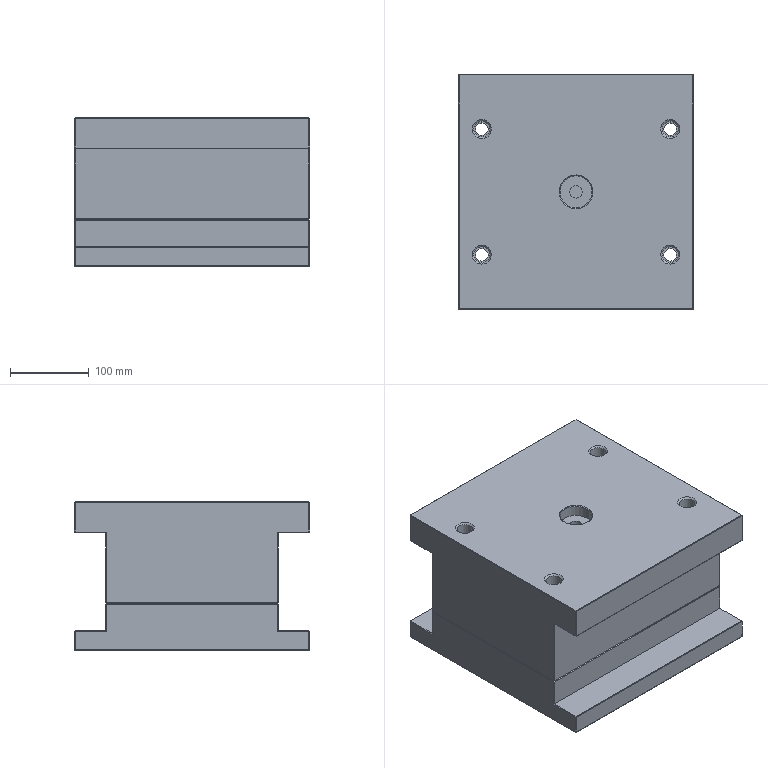NC program | NX | posted with a generic post | part box 300 x 300 x 190 mm
Lines 1 to 721 of 1853:
N10 G17 G21 G94 G90
(HOLE_MILLING_COPY_2 , TOOL : D10C)
N12 T10 M6
N14 G54
N16 G17 G0 G90 X-120. Y80. S2000 M3
N18 G43 Z30. H10
N20 Z0.5
N22 G94 G3 X-117.5 Y77.5 R2.5 F800.
N24 X-115. Y80. R2.5
N26 X-115. Y80. Z0.3 I-5. J0.
N28 X-115. Y80. Z0.1 I-5. J0.
N30 X-115. Y80. Z-0.1 I-5. J0.
N32 X-115. Y80. Z-0.3 I-5. J0.
N34 X-115. Y80. Z-0.5 I-5. J0.
N36 X-115. Y80. Z-0.7 I-5. J0.
N38 X-115. Y80. Z-0.9 I-5. J0.
N40 X-115. Y80. Z-1.1 I-5. J0.
N42 X-115. Y80. Z-1.3 I-5. J0.
N44 X-115. Y80. Z-1.5 I-5. J0.
N46 X-115. Y80. Z-1.7 I-5. J0.
N48 X-115. Y80. Z-1.9 I-5. J0.
N50 X-115. Y80. Z-2.1 I-5. J0.
N52 X-115. Y80. Z-2.3 I-5. J0.
N54 X-115. Y80. Z-2.5 I-5. J0.
N56 X-115. Y80. Z-2.7 I-5. J0.
N58 X-115. Y80. Z-2.9 I-5. J0.
N60 X-115. Y80. Z-3.1 I-5. J0.
N62 X-115. Y80. Z-3.3 I-5. J0.
N64 X-115. Y80. Z-3.5 I-5. J0.
N66 X-115. Y80. Z-3.7 I-5. J0.
N68 X-115. Y80. Z-3.9 I-5. J0.
N70 X-115. Y80. Z-4.1 I-5. J0.
N72 X-115. Y80. Z-4.3 I-5. J0.
N74 X-115. Y80. Z-4.5 I-5. J0.
N76 X-115. Y80. Z-4.7 I-5. J0.
N78 X-115. Y80. Z-4.9 I-5. J0.
N80 X-115. Y80. Z-5.1 I-5. J0.
N82 X-115. Y80. Z-5.3 I-5. J0.
N84 X-115. Y80. Z-5.5 I-5. J0.
N86 X-115. Y80. Z-5.7 I-5. J0.
N88 X-115. Y80. Z-5.9 I-5. J0.
N90 X-115. Y80. Z-6.1 I-5. J0.
N92 X-115. Y80. Z-6.3 I-5. J0.
N94 X-115. Y80. Z-6.5 I-5. J0.
N96 X-115. Y80. Z-6.7 I-5. J0.
N98 X-115. Y80. Z-6.9 I-5. J0.
N100 X-115. Y80. Z-7.1 I-5. J0.
N102 X-115. Y80. Z-7.3 I-5. J0.
N104 X-115. Y80. Z-7.5 I-5. J0.
N106 X-115. Y80. Z-7.7 I-5. J0.
N108 X-115. Y80. Z-7.9 I-5. J0.
N110 X-115. Y80. Z-8.1 I-5. J0.
N112 X-115. Y80. Z-8.3 I-5. J0.
N114 X-115. Y80. Z-8.5 I-5. J0.
N116 X-115. Y80. Z-8.7 I-5. J0.
N118 X-115. Y80. Z-8.9 I-5. J0.
N120 X-115. Y80. Z-9.1 I-5. J0.
N122 X-115. Y80. Z-9.3 I-5. J0.
N124 X-115. Y80. Z-9.5 I-5. J0.
N126 X-115. Y80. Z-9.7 I-5. J0.
N128 X-115. Y80. Z-9.9 I-5. J0.
N130 X-115. Y80. Z-10.1 I-5. J0.
N132 X-115. Y80. Z-10.3 I-5. J0.
N134 X-115. Y80. Z-10.5 I-5. J0.
N136 X-115. Y80. Z-10.7 I-5. J0.
N138 X-115. Y80. Z-10.9 I-5. J0.
N140 X-115. Y80. Z-11.1 I-5. J0.
N142 X-115. Y80. Z-11.3 I-5. J0.
N144 X-115. Y80. Z-11.5 I-5. J0.
N146 X-115. Y80. Z-11.7 I-5. J0.
N148 X-115. Y80. Z-11.9 I-5. J0.
N150 X-115. Y80. Z-12.1 I-5. J0.
N152 X-115. Y80. Z-12.3 I-5. J0.
N154 X-115. Y80. Z-12.5 I-5. J0.
N156 X-115. Y80. Z-12.7 I-5. J0.
N158 X-115. Y80. Z-12.9 I-5. J0.
N160 X-115. Y80. Z-13.1 I-5. J0.
N162 X-115. Y80. Z-13.3 I-5. J0.
N164 X-115. Y80. Z-13.5 I-5. J0.
N166 X-115. Y80. Z-13.7 I-5. J0.
N168 X-115. Y80. Z-13.9 I-5. J0.
N170 X-115. Y80. Z-14.1 I-5. J0.
N172 X-115. Y80. Z-14.3 I-5. J0.
N174 X-115. Y80. Z-14.5 I-5. J0.
N176 X-115. Y80. Z-14.7 I-5. J0.
N178 X-115. Y80. Z-14.9 I-5. J0.
N180 X-115. Y80. Z-15.1 I-5. J0.
N182 X-115. Y80. Z-15.3 I-5. J0.
N184 X-115. Y80. Z-15.5 I-5. J0.
N186 X-115. Y80. Z-15.7 I-5. J0.
N188 X-115. Y80. Z-15.9 I-5. J0.
N190 X-115. Y80. Z-16.1 I-5. J0.
N192 X-115. Y80. Z-16.3 I-5. J0.
N194 X-115. Y80. Z-16.5 I-5. J0.
N196 X-115. Y80. Z-16.7 I-5. J0.
N198 X-115. Y80. Z-16.9 I-5. J0.
N200 X-115. Y80. Z-17.1 I-5. J0.
N202 X-115. Y80. Z-17.3 I-5. J0.
N204 X-115. Y80. Z-17.5 I-5. J0.
N206 X-115. Y80. Z-17.7 I-5. J0.
N208 X-115. Y80. Z-17.9 I-5. J0.
N210 X-115. Y80. Z-18.1 I-5. J0.
N212 X-115. Y80. Z-18.3 I-5. J0.
N214 X-115. Y80. Z-18.5 I-5. J0.
N216 X-115. Y80. Z-18.7 I-5. J0.
N218 X-115. Y80. Z-18.9 I-5. J0.
N220 X-115. Y80. Z-19.1 I-5. J0.
N222 X-115. Y80. Z-19.3 I-5. J0.
N224 X-115. Y80. Z-19.5 I-5. J0.
N226 X-115. Y80. Z-19.7 I-5. J0.
N228 X-115. Y80. Z-19.9 I-5. J0.
N230 X-115. Y80. Z-20.1 I-5. J0.
N232 X-115. Y80. Z-20.3 I-5. J0.
N234 X-115. Y80. Z-20.5 I-5. J0.
N236 X-115. Y80. Z-20.7 I-5. J0.
N238 X-115. Y80. Z-20.9 I-5. J0.
N240 X-115. Y80. Z-21.1 I-5. J0.
N242 X-115. Y80. Z-21.3 I-5. J0.
N244 X-115. Y80. Z-21.5 I-5. J0.
N246 X-115. Y80. Z-21.7 I-5. J0.
N248 X-115. Y80. Z-21.9 I-5. J0.
N250 X-115. Y80. Z-22.1 I-5. J0.
N252 X-115. Y80. Z-22.3 I-5. J0.
N254 X-115. Y80. Z-22.5 I-5. J0.
N256 X-115. Y80. Z-22.7 I-5. J0.
N258 X-115. Y80. Z-22.9 I-5. J0.
N260 X-115. Y80. Z-23.1 I-5. J0.
N262 X-115. Y80. Z-23.3 I-5. J0.
N264 X-115. Y80. Z-23.5 I-5. J0.
N266 X-115. Y80. Z-23.7 I-5. J0.
N268 X-115. Y80. Z-23.9 I-5. J0.
N270 X-115. Y80. Z-24.1 I-5. J0.
N272 X-115. Y80. Z-24.3 I-5. J0.
N274 X-115. Y80. Z-24.5 I-5. J0.
N276 X-115. Y80. Z-24.7 I-5. J0.
N278 X-115. Y80. Z-24.9 I-5. J0.
N280 X-115. Y80. Z-25.1 I-5. J0.
N282 X-115. Y80. Z-25.3 I-5. J0.
N284 X-115. Y80. Z-25.5 I-5. J0.
N286 X-115. Y80. Z-25.7 I-5. J0.
N288 X-115. Y80. Z-25.9 I-5. J0.
N290 X-115. Y80. Z-26.1 I-5. J0.
N292 X-115. Y80. Z-26.3 I-5. J0.
N294 X-115. Y80. Z-26.5 I-5. J0.
N296 X-115. Y80. Z-26.7 I-5. J0.
N298 X-115. Y80. Z-26.9 I-5. J0.
N300 X-115. Y80. Z-27.1 I-5. J0.
N302 X-115. Y80. Z-27.3 I-5. J0.
N304 X-115. Y80. Z-27.5 I-5. J0.
N306 X-115. Y80. Z-27.7 I-5. J0.
N308 X-115. Y80. Z-27.9 I-5. J0.
N310 X-115. Y80. Z-28.1 I-5. J0.
N312 X-115. Y80. Z-28.3 I-5. J0.
N314 X-115. Y80. Z-28.5 I-5. J0.
N316 X-115. Y80. Z-28.7 I-5. J0.
N318 X-115. Y80. Z-28.9 I-5. J0.
N320 X-115. Y80. Z-29.1 I-5. J0.
N322 X-115. Y80. Z-29.3 I-5. J0.
N324 X-115. Y80. Z-29.5 I-5. J0.
N326 X-115. Y80. Z-29.7 I-5. J0.
N328 X-115. Y80. Z-29.9 I-5. J0.
N330 X-115. Y80. Z-30.1 I-5. J0.
N332 X-115. Y80. Z-30.3 I-5. J0.
N334 X-115. Y80. Z-30.5 I-5. J0.
N336 X-115. Y80. Z-30.7 I-5. J0.
N338 X-115. Y80. Z-30.9 I-5. J0.
N340 X-115. Y80. Z-31.1 I-5. J0.
N342 X-115. Y80. Z-31.3 I-5. J0.
N344 X-115. Y80. Z-31.5 I-5. J0.
N346 X-115. Y80. Z-31.7 I-5. J0.
N348 X-115. Y80. Z-31.9 I-5. J0.
N350 X-115. Y80. Z-32.1 I-5. J0.
N352 X-115. Y80. Z-32.3 I-5. J0.
N354 X-115. Y80. Z-32.5 I-5. J0.
N356 X-115. Y80. Z-32.7 I-5. J0.
N358 X-115. Y80. Z-32.9 I-5. J0.
N360 X-115. Y80. Z-33.1 I-5. J0.
N362 X-115. Y80. Z-33.3 I-5. J0.
N364 X-115. Y80. Z-33.5 I-5. J0.
N366 X-115. Y80. Z-33.7 I-5. J0.
N368 X-115. Y80. Z-33.9 I-5. J0.
N370 X-115. Y80. Z-34.1 I-5. J0.
N372 X-115. Y80. Z-34.3 I-5. J0.
N374 X-115. Y80. Z-34.5 I-5. J0.
N376 X-115. Y80. Z-34.7 I-5. J0.
N378 X-115. Y80. Z-34.9 I-5. J0.
N380 X-115. Y80. Z-35.1 I-5. J0.
N382 X-115. Y80. Z-35.3 I-5. J0.
N384 X-115. Y80. Z-35.5 I-5. J0.
N386 X-115. Y80. Z-35.7 I-5. J0.
N388 X-115. Y80. Z-35.9 I-5. J0.
N390 X-115. Y80. Z-36.1 I-5. J0.
N392 X-115. Y80. Z-36.3 I-5. J0.
N394 X-115. Y80. Z-36.5 I-5. J0.
N396 X-115. Y80. Z-36.7 I-5. J0.
N398 X-115. Y80. Z-36.9 I-5. J0.
N400 X-115. Y80. Z-37.1 I-5. J0.
N402 X-115. Y80. Z-37.3 I-5. J0.
N404 X-115. Y80. Z-37.5 I-5. J0.
N406 X-115. Y80. Z-37.7 I-5. J0.
N408 X-115. Y80. Z-37.9 I-5. J0.
N410 X-115. Y80. Z-38.1 I-5. J0.
N412 X-115. Y80. Z-38.3 I-5. J0.
N414 X-115. Y80. Z-38.5 I-5. J0.
N416 X-115. Y80. Z-38.7 I-5. J0.
N418 X-115. Y80. Z-38.9 I-5. J0.
N420 X-115. Y80. Z-39.1 I-5. J0.
N422 X-115. Y80. Z-39.3 I-5. J0.
N424 X-115. Y80. Z-39.5 I-5. J0.
N426 X-115. Y80. Z-39.7 I-5. J0.
N428 X-115. Y80. Z-39.9 I-5. J0.
N430 X-115. Y80. Z-40.1 I-5. J0.
N432 X-115. Y80. Z-40.3 I-5. J0.
N434 X-115. Y80. Z-40.5 I-5. J0.
N436 X-115. Y80. Z-40.7 I-5. J0.
N438 X-115. Y80. Z-40.9 I-5. J0.
N440 X-115. Y80. Z-41.1 I-5. J0.
N442 X-115. Y80. Z-41.3 I-5. J0.
N444 X-115. Y80. Z-41.5 I-5. J0.
N446 X-115. Y80. Z-41.7 I-5. J0.
N448 X-115. Y80. Z-41.9 I-5. J0.
N450 X-115. Y80. Z-42.1 I-5. J0.
N452 X-115. Y80. Z-42.3 I-5. J0.
N454 X-115. Y80. Z-42.5 I-5. J0.
N456 X-115. Y80. Z-42.7 I-5. J0.
N458 X-115. Y80. Z-42.9 I-5. J0.
N460 X-115. Y80. Z-43.1 I-5. J0.
N462 X-115. Y80. Z-43.3 I-5. J0.
N464 X-115. Y80. Z-43.5 I-5. J0.
N466 X-115. Y80. Z-43.7 I-5. J0.
N468 X-115. Y80. Z-43.9 I-5. J0.
N470 X-115. Y80. Z-44.1 I-5. J0.
N472 X-115. Y80. Z-44.3 I-5. J0.
N474 X-115. Y80. Z-44.5 I-5. J0.
N476 X-115. Y80. Z-44.7 I-5. J0.
N478 X-115. Y80. Z-44.9 I-5. J0.
N480 X-115. Y80. Z-45.1 I-5. J0.
N482 X-115. Y80. Z-45.3 I-5. J0.
N484 X-115. Y80. Z-45.5 I-5. J0.
N486 X-115. Y80. Z-45.7 I-5. J0.
N488 X-115. Y80. Z-45.9 I-5. J0.
N490 X-115. Y80. Z-46.1 I-5. J0.
N492 X-115. Y80. Z-46.3 I-5. J0.
N494 X-115. Y80. Z-46.5 I-5. J0.
N496 X-115. Y80. Z-46.7 I-5. J0.
N498 X-115. Y80. Z-46.9 I-5. J0.
N500 X-115. Y80. Z-47.1 I-5. J0.
N502 X-115. Y80. Z-47.3 I-5. J0.
N504 X-115. Y80. Z-47.5 I-5. J0.
N506 X-115. Y80. Z-47.7 I-5. J0.
N508 X-115. Y80. Z-47.9 I-5. J0.
N510 X-115. Y80. Z-48.1 I-5. J0.
N512 X-115. Y80. Z-48.3 I-5. J0.
N514 X-115. Y80. Z-48.5 I-5. J0.
N516 X-115. Y80. Z-48.7 I-5. J0.
N518 X-115. Y80. Z-48.9 I-5. J0.
N520 X-115. Y80. Z-49.1 I-5. J0.
N522 X-115. Y80. Z-49.3 I-5. J0.
N524 X-115. Y80. Z-49.5 I-5. J0.
N526 X-115. Y80. Z-49.7 I-5. J0.
N528 X-115. Y80. Z-49.9 I-5. J0.
N530 X-115. Y80. Z-50.1 I-5. J0.
N532 X-115. Y80. Z-50.3 I-5. J0.
N534 X-115. Y80. Z-50.5 I-5. J0.
N536 X-115. Y80. Z-50.7 I-5. J0.
N538 X-115. Y80. Z-50.9 I-5. J0.
N540 X-115. Y80. Z-51.1 I-5. J0.
N542 X-115. Y80. Z-51.3 I-5. J0.
N544 X-115. Y80. Z-51.5 I-5. J0.
N546 X-115. Y80. Z-51.7 I-5. J0.
N548 X-115. Y80. Z-51.9 I-5. J0.
N550 X-115. Y80. Z-52.1 I-5. J0.
N552 X-115. Y80. Z-52.3 I-5. J0.
N554 X-115. Y80. Z-52.5 I-5. J0.
N556 X-115. Y80. Z-52.7 I-5. J0.
N558 X-115. Y80. Z-52.9 I-5. J0.
N560 X-115. Y80. Z-53.1 I-5. J0.
N562 X-115. Y80. Z-53.3 I-5. J0.
N564 X-115. Y80. Z-53.5 I-5. J0.
N566 X-115. Y80. Z-53.7 I-5. J0.
N568 X-115. Y80. Z-53.9 I-5. J0.
N570 X-115. Y80. Z-54.1 I-5. J0.
N572 X-115. Y80. Z-54.3 I-5. J0.
N574 X-115. Y80. Z-54.5 I-5. J0.
N576 X-115. Y80. Z-54.7 I-5. J0.
N578 X-115. Y80. Z-54.9 I-5. J0.
N580 X-115. Y80. Z-55.1 I-5. J0.
N582 X-115. Y80. Z-55.3 I-5. J0.
N584 X-115. Y80. Z-55.5 I-5. J0.
N586 X-115. Y80. Z-55.7 I-5. J0.
N588 X-115. Y80. Z-55.9 I-5. J0.
N590 X-115. Y80. Z-56.1 I-5. J0.
N592 X-115. Y80. Z-56.3 I-5. J0.
N594 X-115. Y80. Z-56.5 I-5. J0.
N596 X-115. Y80. Z-56.7 I-5. J0.
N598 X-115. Y80. Z-56.9 I-5. J0.
N600 X-115. Y80. Z-57.1 I-5. J0.
N602 X-115. Y80. Z-57.3 I-5. J0.
N604 X-115. Y80. Z-57.5 I-5. J0.
N606 X-115. Y80. Z-57.7 I-5. J0.
N608 X-115. Y80. Z-57.9 I-5. J0.
N610 X-115. Y80. Z-58.1 I-5. J0.
N612 X-115. Y80. Z-58.3 I-5. J0.
N614 X-115. Y80. Z-58.5 I-5. J0.
N616 X-115. Y80. Z-58.7 I-5. J0.
N618 X-115. Y80. Z-58.9 I-5. J0.
N620 X-115. Y80. Z-59.1 I-5. J0.
N622 X-115. Y80. Z-59.3 I-5. J0.
N624 X-115. Y80. Z-59.5 I-5. J0.
N626 X-115. Y80. Z-59.7 I-5. J0.
N628 X-115. Y80. Z-59.9 I-5. J0.
N630 X-115. Y80. Z-60.1 I-5. J0.
N632 X-115. Y80. Z-60.3 I-5. J0.
N634 X-115. Y80. Z-60.5 I-5. J0.
N636 X-115. Y80. Z-60.7 I-5. J0.
N638 X-115. Y80. Z-60.9 I-5. J0.
N640 X-115. Y80. Z-61.1 I-5. J0.
N642 X-115. Y80. Z-61.3 I-5. J0.
N644 X-115. Y80. Z-61.5 I-5. J0.
N646 X-115. Y80. Z-61.7 I-5. J0.
N648 X-115. Y80. Z-61.9 I-5. J0.
N650 X-115. Y80. Z-62.1 I-5. J0.
N652 X-115. Y80. Z-62.3 I-5. J0.
N654 X-115. Y80. Z-62.5 I-5. J0.
N656 X-115. Y80. Z-62.7 I-5. J0.
N658 X-115. Y80. Z-62.9 I-5. J0.
N660 X-115. Y80. Z-63.1 I-5. J0.
N662 X-115. Y80. Z-63.3 I-5. J0.
N664 X-115. Y80. Z-63.5 I-5. J0.
N666 X-115. Y80. Z-63.7 I-5. J0.
N668 X-115. Y80. Z-63.9 I-5. J0.
N670 X-115. Y80. Z-64.1 I-5. J0.
N672 X-115. Y80. Z-64.3 I-5. J0.
N674 X-115. Y80. Z-64.5 I-5. J0.
N676 X-115. Y80. Z-64.7 I-5. J0.
N678 X-115. Y80. Z-64.9 I-5. J0.
N680 X-115. Y80. Z-65.1 I-5. J0.
N682 X-115. Y80. Z-65.3 I-5. J0.
N684 X-115. Y80. Z-65.5 I-5. J0.
N686 X-115. Y80. Z-65.7 I-5. J0.
N688 X-115. Y80. Z-65.9 I-5. J0.
N690 X-115. Y80. Z-66.1 I-5. J0.
N692 X-115. Y80. Z-66.3 I-5. J0.
N694 X-115. Y80. Z-66.5 I-5. J0.
N696 X-115. Y80. Z-66.7 I-5. J0.
N698 X-115. Y80. Z-66.9 I-5. J0.
N700 X-115. Y80. Z-67.1 I-5. J0.
N702 X-115. Y80. Z-67.3 I-5. J0.
N704 X-115. Y80. Z-67.5 I-5. J0.
N706 X-115. Y80. Z-67.7 I-5. J0.
N708 X-115. Y80. Z-67.9 I-5. J0.
N710 X-115. Y80. Z-68.1 I-5. J0.
N712 X-115. Y80. Z-68.3 I-5. J0.
N714 X-115. Y80. Z-68.5 I-5. J0.
N716 X-115. Y80. Z-68.7 I-5. J0.
N718 X-115. Y80. Z-68.9 I-5. J0.
N720 X-115. Y80. Z-69.1 I-5. J0.
N722 X-115. Y80. Z-69.3 I-5. J0.
N724 X-115. Y80. Z-69.5 I-5. J0.
N726 X-115. Y80. Z-69.7 I-5. J0.
N728 X-115. Y80. Z-69.9 I-5. J0.
N730 X-125. Y80. Z-70. I-5. J0.
N732 X-120. Y75. R5.
N734 X-125. Y80. R-5.
N736 X-122.5 Y77.5 R2.5
N738 X-120. Y80. R2.5
N740 G0 Z30.
N742 Y-80.
N744 Z0.5
N746 G3 X-117.5 Y-82.5 R2.5
N748 X-115. Y-80. R2.5
N750 X-115. Y-80. Z0.3 I-5. J0.
N752 X-115. Y-80. Z0.1 I-5. J0.
N754 X-115. Y-80. Z-0.1 I-5. J0.
N756 X-115. Y-80. Z-0.3 I-5. J0.
N758 X-115. Y-80. Z-0.5 I-5. J0.
N760 X-115. Y-80. Z-0.7 I-5. J0.
N762 X-115. Y-80. Z-0.9 I-5. J0.
N764 X-115. Y-80. Z-1.1 I-5. J0.
N766 X-115. Y-80. Z-1.3 I-5. J0.
N768 X-115. Y-80. Z-1.5 I-5. J0.
N770 X-115. Y-80. Z-1.7 I-5. J0.
N772 X-115. Y-80. Z-1.9 I-5. J0.
N774 X-115. Y-80. Z-2.1 I-5. J0.
N776 X-115. Y-80. Z-2.3 I-5. J0.
N778 X-115. Y-80. Z-2.5 I-5. J0.
N780 X-115. Y-80. Z-2.7 I-5. J0.
N782 X-115. Y-80. Z-2.9 I-5. J0.
N784 X-115. Y-80. Z-3.1 I-5. J0.
N786 X-115. Y-80. Z-3.3 I-5. J0.
N788 X-115. Y-80. Z-3.5 I-5. J0.
N790 X-115. Y-80. Z-3.7 I-5. J0.
N792 X-115. Y-80. Z-3.9 I-5. J0.
N794 X-115. Y-80. Z-4.1 I-5. J0.
N796 X-115. Y-80. Z-4.3 I-5. J0.
N798 X-115. Y-80. Z-4.5 I-5. J0.
N800 X-115. Y-80. Z-4.7 I-5. J0.
N802 X-115. Y-80. Z-4.9 I-5. J0.
N804 X-115. Y-80. Z-5.1 I-5. J0.
N806 X-115. Y-80. Z-5.3 I-5. J0.
N808 X-115. Y-80. Z-5.5 I-5. J0.
N810 X-115. Y-80. Z-5.7 I-5. J0.
N812 X-115. Y-80. Z-5.9 I-5. J0.
N814 X-115. Y-80. Z-6.1 I-5. J0.
N816 X-115. Y-80. Z-6.3 I-5. J0.
N818 X-115. Y-80. Z-6.5 I-5. J0.
N820 X-115. Y-80. Z-6.7 I-5. J0.
N822 X-115. Y-80. Z-6.9 I-5. J0.
N824 X-115. Y-80. Z-7.1 I-5. J0.
N826 X-115. Y-80. Z-7.3 I-5. J0.
N828 X-115. Y-80. Z-7.5 I-5. J0.
N830 X-115. Y-80. Z-7.7 I-5. J0.
N832 X-115. Y-80. Z-7.9 I-5. J0.
N834 X-115. Y-80. Z-8.1 I-5. J0.
N836 X-115. Y-80. Z-8.3 I-5. J0.
N838 X-115. Y-80. Z-8.5 I-5. J0.
N840 X-115. Y-80. Z-8.7 I-5. J0.
N842 X-115. Y-80. Z-8.9 I-5. J0.
N844 X-115. Y-80. Z-9.1 I-5. J0.
N846 X-115. Y-80. Z-9.3 I-5. J0.
N848 X-115. Y-80. Z-9.5 I-5. J0.
N850 X-115. Y-80. Z-9.7 I-5. J0.
N852 X-115. Y-80. Z-9.9 I-5. J0.
N854 X-115. Y-80. Z-10.1 I-5. J0.
N856 X-115. Y-80. Z-10.3 I-5. J0.
N858 X-115. Y-80. Z-10.5 I-5. J0.
N860 X-115. Y-80. Z-10.7 I-5. J0.
N862 X-115. Y-80. Z-10.9 I-5. J0.
N864 X-115. Y-80. Z-11.1 I-5. J0.
N866 X-115. Y-80. Z-11.3 I-5. J0.
N868 X-115. Y-80. Z-11.5 I-5. J0.
N870 X-115. Y-80. Z-11.7 I-5. J0.
N872 X-115. Y-80. Z-11.9 I-5. J0.
N874 X-115. Y-80. Z-12.1 I-5. J0.
N876 X-115. Y-80. Z-12.3 I-5. J0.
N878 X-115. Y-80. Z-12.5 I-5. J0.
N880 X-115. Y-80. Z-12.7 I-5. J0.
N882 X-115. Y-80. Z-12.9 I-5. J0.
N884 X-115. Y-80. Z-13.1 I-5. J0.
N886 X-115. Y-80. Z-13.3 I-5. J0.
N888 X-115. Y-80. Z-13.5 I-5. J0.
N890 X-115. Y-80. Z-13.7 I-5. J0.
N892 X-115. Y-80. Z-13.9 I-5. J0.
N894 X-115. Y-80. Z-14.1 I-5. J0.
N896 X-115. Y-80. Z-14.3 I-5. J0.
N898 X-115. Y-80. Z-14.5 I-5. J0.
N900 X-115. Y-80. Z-14.7 I-5. J0.
N902 X-115. Y-80. Z-14.9 I-5. J0.
N904 X-115. Y-80. Z-15.1 I-5. J0.
N906 X-115. Y-80. Z-15.3 I-5. J0.
N908 X-115. Y-80. Z-15.5 I-5. J0.
N910 X-115. Y-80. Z-15.7 I-5. J0.
N912 X-115. Y-80. Z-15.9 I-5. J0.
N914 X-115. Y-80. Z-16.1 I-5. J0.
N916 X-115. Y-80. Z-16.3 I-5. J0.
N918 X-115. Y-80. Z-16.5 I-5. J0.
N920 X-115. Y-80. Z-16.7 I-5. J0.
N922 X-115. Y-80. Z-16.9 I-5. J0.
N924 X-115. Y-80. Z-17.1 I-5. J0.
N926 X-115. Y-80. Z-17.3 I-5. J0.
N928 X-115. Y-80. Z-17.5 I-5. J0.
N930 X-115. Y-80. Z-17.7 I-5. J0.
N932 X-115. Y-80. Z-17.9 I-5. J0.
N934 X-115. Y-80. Z-18.1 I-5. J0.
N936 X-115. Y-80. Z-18.3 I-5. J0.
N938 X-115. Y-80. Z-18.5 I-5. J0.
N940 X-115. Y-80. Z-18.7 I-5. J0.
N942 X-115. Y-80. Z-18.9 I-5. J0.
N944 X-115. Y-80. Z-19.1 I-5. J0.
N946 X-115. Y-80. Z-19.3 I-5. J0.
N948 X-115. Y-80. Z-19.5 I-5. J0.
N950 X-115. Y-80. Z-19.7 I-5. J0.
N952 X-115. Y-80. Z-19.9 I-5. J0.
N954 X-115. Y-80. Z-20.1 I-5. J0.
N956 X-115. Y-80. Z-20.3 I-5. J0.
N958 X-115. Y-80. Z-20.5 I-5. J0.
N960 X-115. Y-80. Z-20.7 I-5. J0.
N962 X-115. Y-80. Z-20.9 I-5. J0.
N964 X-115. Y-80. Z-21.1 I-5. J0.
N966 X-115. Y-80. Z-21.3 I-5. J0.
N968 X-115. Y-80. Z-21.5 I-5. J0.
N970 X-115. Y-80. Z-21.7 I-5. J0.
N972 X-115. Y-80. Z-21.9 I-5. J0.
N974 X-115. Y-80. Z-22.1 I-5. J0.
N976 X-115. Y-80. Z-22.3 I-5. J0.
N978 X-115. Y-80. Z-22.5 I-5. J0.
N980 X-115. Y-80. Z-22.7 I-5. J0.
N982 X-115. Y-80. Z-22.9 I-5. J0.
N984 X-115. Y-80. Z-23.1 I-5. J0.
N986 X-115. Y-80. Z-23.3 I-5. J0.
N988 X-115. Y-80. Z-23.5 I-5. J0.
N990 X-115. Y-80. Z-23.7 I-5. J0.
N992 X-115. Y-80. Z-23.9 I-5. J0.
N994 X-115. Y-80. Z-24.1 I-5. J0.
N996 X-115. Y-80. Z-24.3 I-5. J0.
N998 X-115. Y-80. Z-24.5 I-5. J0.
N1000 X-115. Y-80. Z-24.7 I-5. J0.
N1002 X-115. Y-80. Z-24.9 I-5. J0.
N1004 X-115. Y-80. Z-25.1 I-5. J0.
N1006 X-115. Y-80. Z-25.3 I-5. J0.
N1008 X-115. Y-80. Z-25.5 I-5. J0.
N1010 X-115. Y-80. Z-25.7 I-5. J0.
N1012 X-115. Y-80. Z-25.9 I-5. J0.
N1014 X-115. Y-80. Z-26.1 I-5. J0.
N1016 X-115. Y-80. Z-26.3 I-5. J0.
N1018 X-115. Y-80. Z-26.5 I-5. J0.
N1020 X-115. Y-80. Z-26.7 I-5. J0.
N1022 X-115. Y-80. Z-26.9 I-5. J0.
N1024 X-115. Y-80. Z-27.1 I-5. J0.
N1026 X-115. Y-80. Z-27.3 I-5. J0.
N1028 X-115. Y-80. Z-27.5 I-5. J0.
N1030 X-115. Y-80. Z-27.7 I-5. J0.
N1032 X-115. Y-80. Z-27.9 I-5. J0.
N1034 X-115. Y-80. Z-28.1 I-5. J0.
N1036 X-115. Y-80. Z-28.3 I-5. J0.
N1038 X-115. Y-80. Z-28.5 I-5. J0.
N1040 X-115. Y-80. Z-28.7 I-5. J0.
N1042 X-115. Y-80. Z-28.9 I-5. J0.
N1044 X-115. Y-80. Z-29.1 I-5. J0.
N1046 X-115. Y-80. Z-29.3 I-5. J0.
N1048 X-115. Y-80. Z-29.5 I-5. J0.
N1050 X-115. Y-80. Z-29.7 I-5. J0.
N1052 X-115. Y-80. Z-29.9 I-5. J0.
N1054 X-115. Y-80. Z-30.1 I-5. J0.
N1056 X-115. Y-80. Z-30.3 I-5. J0.
N1058 X-115. Y-80. Z-30.5 I-5. J0.
N1060 X-115. Y-80. Z-30.7 I-5. J0.
N1062 X-115. Y-80. Z-30.9 I-5. J0.
N1064 X-115. Y-80. Z-31.1 I-5. J0.
N1066 X-115. Y-80. Z-31.3 I-5. J0.
N1068 X-115. Y-80. Z-31.5 I-5. J0.
N1070 X-115. Y-80. Z-31.7 I-5. J0.
N1072 X-115. Y-80. Z-31.9 I-5. J0.
N1074 X-115. Y-80. Z-32.1 I-5. J0.
N1076 X-115. Y-80. Z-32.3 I-5. J0.
N1078 X-115. Y-80. Z-32.5 I-5. J0.
N1080 X-115. Y-80. Z-32.7 I-5. J0.
N1082 X-115. Y-80. Z-32.9 I-5. J0.
N1084 X-115. Y-80. Z-33.1 I-5. J0.
N1086 X-115. Y-80. Z-33.3 I-5. J0.
N1088 X-115. Y-80. Z-33.5 I-5. J0.
N1090 X-115. Y-80. Z-33.7 I-5. J0.
N1092 X-115. Y-80. Z-33.9 I-5. J0.
N1094 X-115. Y-80. Z-34.1 I-5. J0.
N1096 X-115. Y-80. Z-34.3 I-5. J0.
N1098 X-115. Y-80. Z-34.5 I-5. J0.
N1100 X-115. Y-80. Z-34.7 I-5. J0.
N1102 X-115. Y-80. Z-34.9 I-5. J0.
N1104 X-115. Y-80. Z-35.1 I-5. J0.
N1106 X-115. Y-80. Z-35.3 I-5. J0.
N1108 X-115. Y-80. Z-35.5 I-5. J0.
N1110 X-115. Y-80. Z-35.7 I-5. J0.
N1112 X-115. Y-80. Z-35.9 I-5. J0.
N1114 X-115. Y-80. Z-36.1 I-5. J0.
N1116 X-115. Y-80. Z-36.3 I-5. J0.
N1118 X-115. Y-80. Z-36.5 I-5. J0.
N1120 X-115. Y-80. Z-36.7 I-5. J0.
N1122 X-115. Y-80. Z-36.9 I-5. J0.
N1124 X-115. Y-80. Z-37.1 I-5. J0.
N1126 X-115. Y-80. Z-37.3 I-5. J0.
N1128 X-115. Y-80. Z-37.5 I-5. J0.
N1130 X-115. Y-80. Z-37.7 I-5. J0.
N1132 X-115. Y-80. Z-37.9 I-5. J0.
N1134 X-115. Y-80. Z-38.1 I-5. J0.
N1136 X-115. Y-80. Z-38.3 I-5. J0.
N1138 X-115. Y-80. Z-38.5 I-5. J0.
N1140 X-115. Y-80. Z-38.7 I-5. J0.
N1142 X-115. Y-80. Z-38.9 I-5. J0.
N1144 X-115. Y-80. Z-39.1 I-5. J0.
N1146 X-115. Y-80. Z-39.3 I-5. J0.
N1148 X-115. Y-80. Z-39.5 I-5. J0.
N1150 X-115. Y-80. Z-39.7 I-5. J0.
N1152 X-115. Y-80. Z-39.9 I-5. J0.
N1154 X-115. Y-80. Z-40.1 I-5. J0.
N1156 X-115. Y-80. Z-40.3 I-5. J0.
N1158 X-115. Y-80. Z-40.5 I-5. J0.
N1160 X-115. Y-80. Z-40.7 I-5. J0.
N1162 X-115. Y-80. Z-40.9 I-5. J0.
N1164 X-115. Y-80. Z-41.1 I-5. J0.
N1166 X-115. Y-80. Z-41.3 I-5. J0.
N1168 X-115. Y-80. Z-41.5 I-5. J0.
N1170 X-115. Y-80. Z-41.7 I-5. J0.
N1172 X-115. Y-80. Z-41.9 I-5. J0.
N1174 X-115. Y-80. Z-42.1 I-5. J0.
N1176 X-115. Y-80. Z-42.3 I-5. J0.
N1178 X-115. Y-80. Z-42.5 I-5. J0.
N1180 X-115. Y-80. Z-42.7 I-5. J0.
N1182 X-115. Y-80. Z-42.9 I-5. J0.
N1184 X-115. Y-80. Z-43.1 I-5. J0.
N1186 X-115. Y-80. Z-43.3 I-5. J0.
N1188 X-115. Y-80. Z-43.5 I-5. J0.
N1190 X-115. Y-80. Z-43.7 I-5. J0.
N1192 X-115. Y-80. Z-43.9 I-5. J0.
N1194 X-115. Y-80. Z-44.1 I-5. J0.
N1196 X-115. Y-80. Z-44.3 I-5. J0.
N1198 X-115. Y-80. Z-44.5 I-5. J0.
N1200 X-115. Y-80. Z-44.7 I-5. J0.
N1202 X-115. Y-80. Z-44.9 I-5. J0.
N1204 X-115. Y-80. Z-45.1 I-5. J0.
N1206 X-115. Y-80. Z-45.3 I-5. J0.
N1208 X-115. Y-80. Z-45.5 I-5. J0.
N1210 X-115. Y-80. Z-45.7 I-5. J0.
N1212 X-115. Y-80. Z-45.9 I-5. J0.
N1214 X-115. Y-80. Z-46.1 I-5. J0.
N1216 X-115. Y-80. Z-46.3 I-5. J0.
N1218 X-115. Y-80. Z-46.5 I-5. J0.
N1220 X-115. Y-80. Z-46.7 I-5. J0.
N1222 X-115. Y-80. Z-46.9 I-5. J0.
N1224 X-115. Y-80. Z-47.1 I-5. J0.
N1226 X-115. Y-80. Z-47.3 I-5. J0.
N1228 X-115. Y-80. Z-47.5 I-5. J0.
N1230 X-115. Y-80. Z-47.7 I-5. J0.
N1232 X-115. Y-80. Z-47.9 I-5. J0.
N1234 X-115. Y-80. Z-48.1 I-5. J0.
N1236 X-115. Y-80. Z-48.3 I-5. J0.
N1238 X-115. Y-80. Z-48.5 I-5. J0.
N1240 X-115. Y-80. Z-48.7 I-5. J0.
N1242 X-115. Y-80. Z-48.9 I-5. J0.
N1244 X-115. Y-80. Z-49.1 I-5. J0.
N1246 X-115. Y-80. Z-49.3 I-5. J0.
N1248 X-115. Y-80. Z-49.5 I-5. J0.
N1250 X-115. Y-80. Z-49.7 I-5. J0.
N1252 X-115. Y-80. Z-49.9 I-5. J0.
N1254 X-115. Y-80. Z-50.1 I-5. J0.
N1256 X-115. Y-80. Z-50.3 I-5. J0.
N1258 X-115. Y-80. Z-50.5 I-5. J0.
N1260 X-115. Y-80. Z-50.7 I-5. J0.
N1262 X-115. Y-80. Z-50.9 I-5. J0.
N1264 X-115. Y-80. Z-51.1 I-5. J0.
N1266 X-115. Y-80. Z-51.3 I-5. J0.
N1268 X-115. Y-80. Z-51.5 I-5. J0.
N1270 X-115. Y-80. Z-51.7 I-5. J0.
N1272 X-115. Y-80. Z-51.9 I-5. J0.
N1274 X-115. Y-80. Z-52.1 I-5. J0.
N1276 X-115. Y-80. Z-52.3 I-5. J0.
N1278 X-115. Y-80. Z-52.5 I-5. J0.
N1280 X-115. Y-80. Z-52.7 I-5. J0.
N1282 X-115. Y-80. Z-52.9 I-5. J0.
N1284 X-115. Y-80. Z-53.1 I-5. J0.
N1286 X-115. Y-80. Z-53.3 I-5. J0.
N1288 X-115. Y-80. Z-53.5 I-5. J0.
N1290 X-115. Y-80. Z-53.7 I-5. J0.
N1292 X-115. Y-80. Z-53.9 I-5. J0.
N1294 X-115. Y-80. Z-54.1 I-5. J0.
N1296 X-115. Y-80. Z-54.3 I-5. J0.
N1298 X-115. Y-80. Z-54.5 I-5. J0.
N1300 X-115. Y-80. Z-54.7 I-5. J0.
N1302 X-115. Y-80. Z-54.9 I-5. J0.
N1304 X-115. Y-80. Z-55.1 I-5. J0.
N1306 X-115. Y-80. Z-55.3 I-5. J0.
N1308 X-115. Y-80. Z-55.5 I-5. J0.
N1310 X-115. Y-80. Z-55.7 I-5. J0.
N1312 X-115. Y-80. Z-55.9 I-5. J0.
N1314 X-115. Y-80. Z-56.1 I-5. J0.
N1316 X-115. Y-80. Z-56.3 I-5. J0.
N1318 X-115. Y-80. Z-56.5 I-5. J0.
N1320 X-115. Y-80. Z-56.7 I-5. J0.
N1322 X-115. Y-80. Z-56.9 I-5. J0.
N1324 X-115. Y-80. Z-57.1 I-5. J0.
N1326 X-115. Y-80. Z-57.3 I-5. J0.
N1328 X-115. Y-80. Z-57.5 I-5. J0.
N1330 X-115. Y-80. Z-57.7 I-5. J0.
N1332 X-115. Y-80. Z-57.9 I-5. J0.
N1334 X-115. Y-80. Z-58.1 I-5. J0.
N1336 X-115. Y-80. Z-58.3 I-5. J0.
N1338 X-115. Y-80. Z-58.5 I-5. J0.
N1340 X-115. Y-80. Z-58.7 I-5. J0.
N1342 X-115. Y-80. Z-58.9 I-5. J0.
N1344 X-115. Y-80. Z-59.1 I-5. J0.
N1346 X-115. Y-80. Z-59.3 I-5. J0.
N1348 X-115. Y-80. Z-59.5 I-5. J0.
N1350 X-115. Y-80. Z-59.7 I-5. J0.
N1352 X-115. Y-80. Z-59.9 I-5. J0.
N1354 X-115. Y-80. Z-60.1 I-5. J0.
N1356 X-115. Y-80. Z-60.3 I-5. J0.
N1358 X-115. Y-80. Z-60.5 I-5. J0.
N1360 X-115. Y-80. Z-60.7 I-5. J0.
N1362 X-115. Y-80. Z-60.9 I-5. J0.
N1364 X-115. Y-80. Z-61.1 I-5. J0.
N1366 X-115. Y-80. Z-61.3 I-5. J0.
N1368 X-115. Y-80. Z-61.5 I-5. J0.
N1370 X-115. Y-80. Z-61.7 I-5. J0.
N1372 X-115. Y-80. Z-61.9 I-5. J0.
N1374 X-115. Y-80. Z-62.1 I-5. J0.
N1376 X-115. Y-80. Z-62.3 I-5. J0.
N1378 X-115. Y-80. Z-62.5 I-5. J0.
N1380 X-115. Y-80. Z-62.7 I-5. J0.
N1382 X-115. Y-80. Z-62.9 I-5. J0.
N1384 X-115. Y-80. Z-63.1 I-5. J0.
N1386 X-115. Y-80. Z-63.3 I-5. J0.
N1388 X-115. Y-80. Z-63.5 I-5. J0.
N1390 X-115. Y-80. Z-63.7 I-5. J0.
N1392 X-115. Y-80. Z-63.9 I-5. J0.
N1394 X-115. Y-80. Z-64.1 I-5. J0.
N1396 X-115. Y-80. Z-64.3 I-5. J0.
N1398 X-115. Y-80. Z-64.5 I-5. J0.
N1400 X-115. Y-80. Z-64.7 I-5. J0.
N1402 X-115. Y-80. Z-64.9 I-5. J0.
N1404 X-115. Y-80. Z-65.1 I-5. J0.
N1406 X-115. Y-80. Z-65.3 I-5. J0.
N1408 X-115. Y-80. Z-65.5 I-5. J0.
N1410 X-115. Y-80. Z-65.7 I-5. J0.
N1412 X-115. Y-80. Z-65.9 I-5. J0.
N1414 X-115. Y-80. Z-66.1 I-5. J0.
N1416 X-115. Y-80. Z-66.3 I-5. J0.
N1418 X-115. Y-80. Z-66.5 I-5. J0.
N1420 X-115. Y-80. Z-66.7 I-5. J0.
N1422 X-115. Y-80. Z-66.9 I-5. J0.
N1424 X-115. Y-80. Z-67.1 I-5. J0.
N1426 X-115. Y-80. Z-67.3 I-5. J0.
N1428 X-115. Y-80. Z-67.5 I-5. J0.
N1430 X-115. Y-80. Z-67.7 I-5. J0.
N1432 X-115. Y-80. Z-67.9 I-5. J0.
N1434 X-115. Y-80. Z-68.1 I-5. J0.
N1436 X-115. Y-80. Z-68.3 I-5. J0.
N1438 X-115. Y-80. Z-68.5 I-5. J0.
N1440 X-115. Y-80. Z-68.7 I-5. J0.